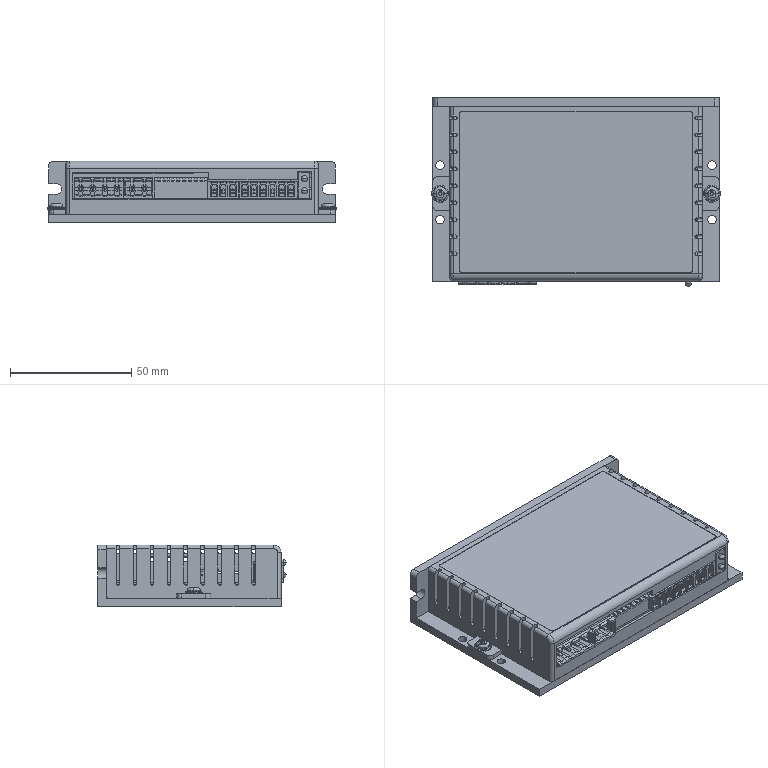Part | STEP file | Stepper motor driver DM542-KK V3.0 | 15 solids | 1923 faces | box 119 x 77.6 x 25.5 mm | volume 99944 mm3 | plane 1518 | cylinder 349 | cone 28 | torus 18 | spline 4 | sphere 4 | other 2 | commonest cylinder face diameters 1.5 x92 3 x80 2.35 x34 2.032 x30 2 x22 3.5 x16